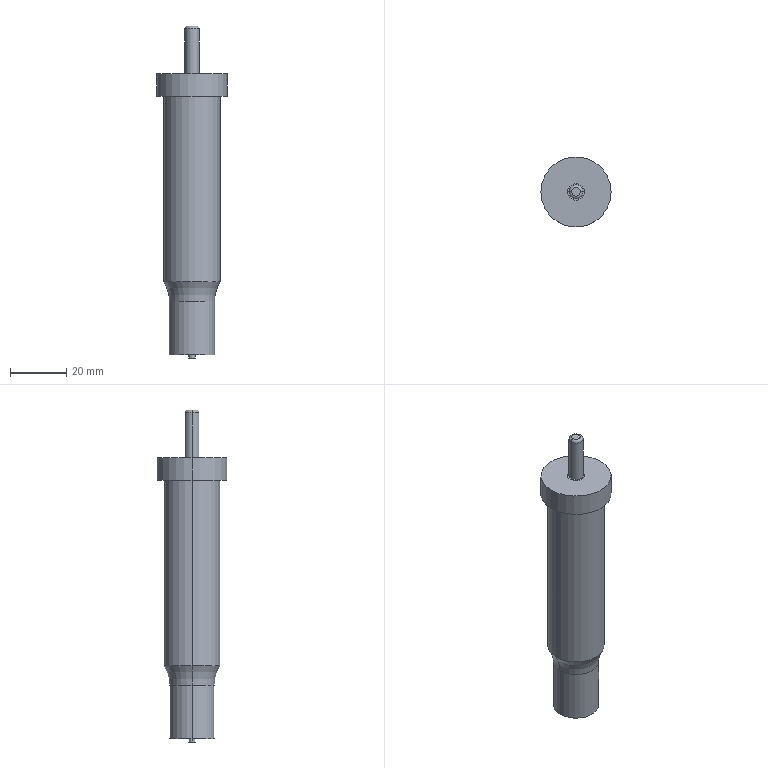Part | STEP file | 1_id3662_x_t | 1 solid | 22 faces | box 25 x 25 x 118.2 mm | volume 30521 mm3 | cylinder 12 | plane 6 | torus 4 | commonest cylinder face diameters 2.26 x2 5 x2 6 x2 16.07 x2 20 x2 25 x2
STEP:
#1=CARTESIAN_POINT('',(3377.,75.5,84.5));
#2=VERTEX_POINT('',#1);
#3=CARTESIAN_POINT('',(3377.,75.5,92.5));
#4=VERTEX_POINT('',#3);
#5=CARTESIAN_POINT('',(3377.,75.5,88.5));
#6=DIRECTION('',(0.,0.,1.));
#7=VECTOR('',#6,1.);
#8=LINE('',#5,#7);
#9=EDGE_CURVE('',#2,#4,#8,.T.);
#10=ORIENTED_EDGE('',*,*,#9,.F.);
#11=CARTESIAN_POINT('',(3352.,75.5,84.5));
#12=VERTEX_POINT('',#11);
#13=CARTESIAN_POINT('',(3364.5,75.5,84.5));
#14=DIRECTION('',(0.,0.,1.));
#15=DIRECTION('',(1.,0.,0.));
#16=AXIS2_PLACEMENT_3D('',#13,#14,#15);
#17=CIRCLE('',#16,12.5);
#18=EDGE_CURVE('',#2,#12,#17,.T.);
#19=ORIENTED_EDGE('',*,*,#18,.T.);
#20=CARTESIAN_POINT('',(3352.,75.5,92.5));
#21=VERTEX_POINT('',#20);
#22=CARTESIAN_POINT('',(3352.,75.5,88.5));
#23=DIRECTION('',(0.,0.,-1.));
#24=VECTOR('',#23,1.);
#25=LINE('',#22,#24);
#26=EDGE_CURVE('',#21,#12,#25,.T.);
#27=ORIENTED_EDGE('',*,*,#26,.F.);
#28=CARTESIAN_POINT('',(3364.5,75.5,92.5));
#29=DIRECTION('',(0.,0.,1.));
#30=DIRECTION('',(1.,0.,0.));
#31=AXIS2_PLACEMENT_3D('',#28,#29,#30);
#32=CIRCLE('',#31,12.5);
#33=EDGE_CURVE('',#4,#21,#32,.T.);
#34=ORIENTED_EDGE('',*,*,#33,.F.);
#35=EDGE_LOOP('',(#10,#19,#27,#34));
#36=FACE_OUTER_BOUND('',#35,.T.);
#37=CARTESIAN_POINT('',(3364.5,75.5,88.5));
#38=DIRECTION('',(0.,0.,-1.));
#39=DIRECTION('',(-1.,0.,0.));
#40=AXIS2_PLACEMENT_3D('',#37,#38,#39);
#41=CYLINDRICAL_SURFACE('',#40,12.5);
#42=ADVANCED_FACE('',(#36),#41,.T.);
#43=CARTESIAN_POINT('',(3374.5,75.5,18.372));
#44=VERTEX_POINT('',#43);
#45=CARTESIAN_POINT('',(3374.5,75.5,84.5));
#46=VERTEX_POINT('',#45);
#47=CARTESIAN_POINT('',(3374.5,75.5,38.5));
#48=DIRECTION('',(0.,0.,1.));
#49=VECTOR('',#48,1.);
#50=LINE('',#47,#49);
#51=EDGE_CURVE('',#44,#46,#50,.T.);
#52=ORIENTED_EDGE('',*,*,#51,.F.);
#53=CARTESIAN_POINT('',(3354.5,75.5,18.372));
#54=VERTEX_POINT('',#53);
#55=CARTESIAN_POINT('',(3364.5,75.5,18.372));
#56=DIRECTION('',(0.,0.,1.));
#57=DIRECTION('',(1.,0.,0.));
#58=AXIS2_PLACEMENT_3D('',#55,#56,#57);
#59=CIRCLE('',#58,10.);
#60=EDGE_CURVE('',#44,#54,#59,.T.);
#61=ORIENTED_EDGE('',*,*,#60,.T.);
#62=CARTESIAN_POINT('',(3354.5,75.5,84.5));
#63=VERTEX_POINT('',#62);
#64=CARTESIAN_POINT('',(3354.5,75.5,38.5));
#65=DIRECTION('',(0.,0.,-1.));
#66=VECTOR('',#65,1.);
#67=LINE('',#64,#66);
#68=EDGE_CURVE('',#63,#54,#67,.T.);
#69=ORIENTED_EDGE('',*,*,#68,.F.);
#70=CARTESIAN_POINT('',(3364.5,75.5,84.5));
#71=DIRECTION('',(0.,0.,1.));
#72=DIRECTION('',(1.,0.,0.));
#73=AXIS2_PLACEMENT_3D('',#70,#71,#72);
#74=CIRCLE('',#73,10.);
#75=EDGE_CURVE('',#46,#63,#74,.T.);
#76=ORIENTED_EDGE('',*,*,#75,.F.);
#77=EDGE_LOOP('',(#52,#61,#69,#76));
#78=FACE_OUTER_BOUND('',#77,.T.);
#79=CARTESIAN_POINT('',(3364.5,75.5,38.5));
#80=DIRECTION('',(0.,0.,-1.));
#81=DIRECTION('',(-1.,0.,0.));
#82=AXIS2_PLACEMENT_3D('',#79,#80,#81);
#83=CYLINDRICAL_SURFACE('',#82,10.);
#84=ADVANCED_FACE('',(#78),#83,.T.);
#85=CARTESIAN_POINT('',(3372.535,75.5,11.5));
#86=VERTEX_POINT('',#85);
#87=CARTESIAN_POINT('',(3372.535,75.5,-7.5));
#88=VERTEX_POINT('',#87);
#89=CARTESIAN_POINT('',(3372.535,75.5,2.));
#90=DIRECTION('',(0.,0.,-1.));
#91=VECTOR('',#90,1.);
#92=LINE('',#89,#91);
#93=EDGE_CURVE('',#86,#88,#92,.T.);
#94=ORIENTED_EDGE('',*,*,#93,.F.);
#95=CARTESIAN_POINT('',(3356.465,75.5,11.5));
#96=VERTEX_POINT('',#95);
#97=CARTESIAN_POINT('',(3364.5,75.5,11.5));
#98=DIRECTION('',(0.,0.,1.));
#99=DIRECTION('',(1.,0.,0.));
#100=AXIS2_PLACEMENT_3D('',#97,#98,#99);
#101=CIRCLE('',#100,8.035);
#102=EDGE_CURVE('',#96,#86,#101,.T.);
#103=ORIENTED_EDGE('',*,*,#102,.F.);
#104=CARTESIAN_POINT('',(3356.465,75.5,-7.5));
#105=VERTEX_POINT('',#104);
#106=CARTESIAN_POINT('',(3356.465,75.5,2.));
#107=DIRECTION('',(0.,0.,1.));
#108=VECTOR('',#107,1.);
#109=LINE('',#106,#108);
#110=EDGE_CURVE('',#105,#96,#109,.T.);
#111=ORIENTED_EDGE('',*,*,#110,.F.);
#112=CARTESIAN_POINT('',(3364.5,75.5,-7.5));
#113=DIRECTION('',(0.,0.,-1.));
#114=DIRECTION('',(1.,0.,0.));
#115=AXIS2_PLACEMENT_3D('',#112,#113,#114);
#116=CIRCLE('',#115,8.035);
#117=EDGE_CURVE('',#88,#105,#116,.T.);
#118=ORIENTED_EDGE('',*,*,#117,.F.);
#119=EDGE_LOOP('',(#94,#103,#111,#118));
#120=FACE_OUTER_BOUND('',#119,.T.);
#121=CARTESIAN_POINT('',(3364.5,75.5,2.));
#122=DIRECTION('',(0.,0.,-1.));
#123=DIRECTION('',(-1.,0.,0.));
#124=AXIS2_PLACEMENT_3D('',#121,#122,#123);
#125=CYLINDRICAL_SURFACE('',#124,8.035);
#126=ADVANCED_FACE('',(#120),#125,.T.);
#127=CARTESIAN_POINT('',(3343.465,75.5,11.5));
#128=DIRECTION('',(0.,-1.,0.));
#129=DIRECTION('',(-1.,0.,0.));
#130=AXIS2_PLACEMENT_3D('',#127,#128,#129);
#131=CIRCLE('',#130,13.);
#132=EDGE_CURVE('',#96,#54,#131,.T.);
#133=ORIENTED_EDGE('',*,*,#132,.F.);
#134=ORIENTED_EDGE('',*,*,#102,.T.);
#135=CARTESIAN_POINT('',(3385.535,75.5,11.5));
#136=DIRECTION('',(0.,-1.,0.));
#137=DIRECTION('',(1.,0.,0.));
#138=AXIS2_PLACEMENT_3D('',#135,#136,#137);
#139=CIRCLE('',#138,13.);
#140=EDGE_CURVE('',#44,#86,#139,.T.);
#141=ORIENTED_EDGE('',*,*,#140,.F.);
#142=CARTESIAN_POINT('',(3364.5,75.5,18.372));
#143=DIRECTION('',(0.,0.,1.));
#144=DIRECTION('',(1.,0.,0.));
#145=AXIS2_PLACEMENT_3D('',#142,#143,#144);
#146=CIRCLE('',#145,10.);
#147=EDGE_CURVE('',#54,#44,#146,.T.);
#148=ORIENTED_EDGE('',*,*,#147,.F.);
#149=EDGE_LOOP('',(#133,#134,#141,#148));
#150=FACE_OUTER_BOUND('',#149,.T.);
#151=CARTESIAN_POINT('',(3364.5,75.5,11.5));
#152=DIRECTION('',(0.,0.,1.));
#153=DIRECTION('',(1.,0.,0.));
#154=AXIS2_PLACEMENT_3D('',#151,#152,#153);
#155=TOROIDAL_SURFACE('',#154,21.035,13.);
#156=ADVANCED_FACE('',(#150),#155,.F.);
#157=CARTESIAN_POINT('',(3363.37,75.5,-7.5));
#158=VERTEX_POINT('',#157);
#159=CARTESIAN_POINT('',(3363.37,75.5,-8.7));
#160=VERTEX_POINT('',#159);
#161=CARTESIAN_POINT('',(3363.37,75.5,-7.5));
#162=DIRECTION('',(0.,0.,-1.));
#163=VECTOR('',#162,1.);
#164=LINE('',#161,#163);
#165=EDGE_CURVE('',#158,#160,#164,.T.);
#166=ORIENTED_EDGE('',*,*,#165,.F.);
#167=CARTESIAN_POINT('',(3365.63,75.5,-7.5));
#168=VERTEX_POINT('',#167);
#169=CARTESIAN_POINT('',(3364.5,75.5,-7.5));
#170=DIRECTION('',(0.,0.,1.));
#171=DIRECTION('',(-1.,0.,0.));
#172=AXIS2_PLACEMENT_3D('',#169,#170,#171);
#173=CIRCLE('',#172,1.13);
#174=EDGE_CURVE('',#168,#158,#173,.T.);
#175=ORIENTED_EDGE('',*,*,#174,.F.);
#176=CARTESIAN_POINT('',(3365.63,75.5,-8.7));
#177=VERTEX_POINT('',#176);
#178=CARTESIAN_POINT('',(3365.63,75.5,-7.5));
#179=DIRECTION('',(0.,0.,1.));
#180=VECTOR('',#179,1.);
#181=LINE('',#178,#180);
#182=EDGE_CURVE('',#177,#168,#181,.T.);
#183=ORIENTED_EDGE('',*,*,#182,.F.);
#184=CARTESIAN_POINT('',(3364.5,75.5,-8.7));
#185=DIRECTION('',(0.,0.,1.));
#186=DIRECTION('',(-1.,0.,0.));
#187=AXIS2_PLACEMENT_3D('',#184,#185,#186);
#188=CIRCLE('',#187,1.13);
#189=EDGE_CURVE('',#177,#160,#188,.T.);
#190=ORIENTED_EDGE('',*,*,#189,.T.);
#191=EDGE_LOOP('',(#166,#175,#183,#190));
#192=FACE_OUTER_BOUND('',#191,.T.);
#193=CARTESIAN_POINT('',(3364.5,75.5,-7.5));
#194=DIRECTION('',(0.,0.,1.));
#195=DIRECTION('',(1.,0.,0.));
#196=AXIS2_PLACEMENT_3D('',#193,#194,#195);
#197=CYLINDRICAL_SURFACE('',#196,1.13);
#198=ADVANCED_FACE('',(#192),#197,.T.);
#199=CARTESIAN_POINT('',(3362.,75.5,108.5));
#200=VERTEX_POINT('',#199);
#201=CARTESIAN_POINT('',(3362.,75.5,92.6));
#202=VERTEX_POINT('',#201);
#203=CARTESIAN_POINT('',(3362.,75.5,100.55));
#204=DIRECTION('',(0.,0.,-1.));
#205=VECTOR('',#204,1.);
#206=LINE('',#203,#205);
#207=EDGE_CURVE('',#200,#202,#206,.T.);
#208=ORIENTED_EDGE('',*,*,#207,.F.);
#209=CARTESIAN_POINT('',(3367.,75.5,108.5));
#210=VERTEX_POINT('',#209);
#211=CARTESIAN_POINT('',(3364.5,75.5,108.5));
#212=DIRECTION('',(0.,0.,-1.));
#213=DIRECTION('',(-1.,0.,0.));
#214=AXIS2_PLACEMENT_3D('',#211,#212,#213);
#215=CIRCLE('',#214,2.5);
#216=EDGE_CURVE('',#200,#210,#215,.T.);
#217=ORIENTED_EDGE('',*,*,#216,.T.);
#218=CARTESIAN_POINT('',(3367.,75.5,92.6));
#219=VERTEX_POINT('',#218);
#220=CARTESIAN_POINT('',(3367.,75.5,100.55));
#221=DIRECTION('',(0.,0.,1.));
#222=VECTOR('',#221,1.);
#223=LINE('',#220,#222);
#224=EDGE_CURVE('',#219,#210,#223,.T.);
#225=ORIENTED_EDGE('',*,*,#224,.F.);
#226=CARTESIAN_POINT('',(3364.5,75.5,92.6));
#227=DIRECTION('',(0.,0.,-1.));
#228=DIRECTION('',(-1.,0.,0.));
#229=AXIS2_PLACEMENT_3D('',#226,#227,#228);
#230=CIRCLE('',#229,2.5);
#231=EDGE_CURVE('',#202,#219,#230,.T.);
#232=ORIENTED_EDGE('',*,*,#231,.F.);
#233=EDGE_LOOP('',(#208,#217,#225,#232));
#234=FACE_OUTER_BOUND('',#233,.T.);
#235=CARTESIAN_POINT('',(3364.5,75.5,100.55));
#236=DIRECTION('',(0.,0.,1.));
#237=DIRECTION('',(1.,0.,0.));
#238=AXIS2_PLACEMENT_3D('',#235,#236,#237);
#239=CYLINDRICAL_SURFACE('',#238,2.5);
#240=ADVANCED_FACE('',(#234),#239,.T.);
#241=CARTESIAN_POINT('',(3366.,75.5,109.5));
#242=VERTEX_POINT('',#241);
#243=CARTESIAN_POINT('',(3366.,75.5,108.5));
#244=DIRECTION('',(0.,1.,0.));
#245=DIRECTION('',(1.,0.,0.));
#246=AXIS2_PLACEMENT_3D('',#243,#244,#245);
#247=CIRCLE('',#246,1.);
#248=EDGE_CURVE('',#242,#210,#247,.T.);
#249=ORIENTED_EDGE('',*,*,#248,.F.);
#250=CARTESIAN_POINT('',(3363.,75.5,109.5));
#251=VERTEX_POINT('',#250);
#252=CARTESIAN_POINT('',(3364.5,75.5,109.5));
#253=DIRECTION('',(0.,0.,-1.));
#254=DIRECTION('',(-1.,0.,0.));
#255=AXIS2_PLACEMENT_3D('',#252,#253,#254);
#256=CIRCLE('',#255,1.5);
#257=EDGE_CURVE('',#242,#251,#256,.T.);
#258=ORIENTED_EDGE('',*,*,#257,.T.);
#259=CARTESIAN_POINT('',(3363.,75.5,108.5));
#260=DIRECTION('',(0.,1.,0.));
#261=DIRECTION('',(-1.,0.,0.));
#262=AXIS2_PLACEMENT_3D('',#259,#260,#261);
#263=CIRCLE('',#262,1.);
#264=EDGE_CURVE('',#200,#251,#263,.T.);
#265=ORIENTED_EDGE('',*,*,#264,.F.);
#266=CARTESIAN_POINT('',(3364.5,75.5,108.5));
#267=DIRECTION('',(0.,0.,-1.));
#268=DIRECTION('',(-1.,0.,0.));
#269=AXIS2_PLACEMENT_3D('',#266,#267,#268);
#270=CIRCLE('',#269,2.5);
#271=EDGE_CURVE('',#210,#200,#270,.T.);
#272=ORIENTED_EDGE('',*,*,#271,.F.);
#273=EDGE_LOOP('',(#249,#258,#265,#272));
#274=FACE_OUTER_BOUND('',#273,.T.);
#275=CARTESIAN_POINT('',(3364.5,75.5,108.5));
#276=DIRECTION('',(0.,0.,-1.));
#277=DIRECTION('',(-1.,0.,0.));
#278=AXIS2_PLACEMENT_3D('',#275,#276,#277);
#279=TOROIDAL_SURFACE('',#278,1.5,1.);
#280=ADVANCED_FACE('',(#274),#279,.T.);
#281=CARTESIAN_POINT('',(3361.5,75.5,92.6));
#282=VERTEX_POINT('',#281);
#283=CARTESIAN_POINT('',(3361.5,75.5,92.5));
#284=VERTEX_POINT('',#283);
#285=CARTESIAN_POINT('',(3361.5,75.5,92.55));
#286=DIRECTION('',(0.,0.,-1.));
#287=VECTOR('',#286,1.);
#288=LINE('',#285,#287);
#289=EDGE_CURVE('',#282,#284,#288,.T.);
#290=ORIENTED_EDGE('',*,*,#289,.F.);
#291=CARTESIAN_POINT('',(3367.5,75.5,92.6));
#292=VERTEX_POINT('',#291);
#293=CARTESIAN_POINT('',(3364.5,75.5,92.6));
#294=DIRECTION('',(0.,0.,-1.));
#295=DIRECTION('',(-1.,0.,0.));
#296=AXIS2_PLACEMENT_3D('',#293,#294,#295);
#297=CIRCLE('',#296,3.);
#298=EDGE_CURVE('',#282,#292,#297,.T.);
#299=ORIENTED_EDGE('',*,*,#298,.T.);
#300=CARTESIAN_POINT('',(3367.5,75.5,92.5));
#301=VERTEX_POINT('',#300);
#302=CARTESIAN_POINT('',(3367.5,75.5,92.55));
#303=DIRECTION('',(0.,0.,1.));
#304=VECTOR('',#303,1.);
#305=LINE('',#302,#304);
#306=EDGE_CURVE('',#301,#292,#305,.T.);
#307=ORIENTED_EDGE('',*,*,#306,.F.);
#308=CARTESIAN_POINT('',(3364.5,75.5,92.5));
#309=DIRECTION('',(0.,0.,-1.));
#310=DIRECTION('',(-1.,0.,0.));
#311=AXIS2_PLACEMENT_3D('',#308,#309,#310);
#312=CIRCLE('',#311,3.);
#313=EDGE_CURVE('',#284,#301,#312,.T.);
#314=ORIENTED_EDGE('',*,*,#313,.F.);
#315=EDGE_LOOP('',(#290,#299,#307,#314));
#316=FACE_OUTER_BOUND('',#315,.T.);
#317=CARTESIAN_POINT('',(3364.5,75.5,87.05));
#318=DIRECTION('',(0.,0.,1.));
#319=DIRECTION('',(1.,0.,0.));
#320=AXIS2_PLACEMENT_3D('',#317,#318,#319);
#321=CYLINDRICAL_SURFACE('',#320,3.);
#322=ADVANCED_FACE('',(#316),#321,.T.);
#323=ORIENTED_EDGE('',*,*,#289,.T.);
#324=CARTESIAN_POINT('',(3364.5,75.5,92.5));
#325=DIRECTION('',(0.,0.,-1.));
#326=DIRECTION('',(-1.,0.,0.));
#327=AXIS2_PLACEMENT_3D('',#324,#325,#326);
#328=CIRCLE('',#327,3.);
#329=EDGE_CURVE('',#301,#284,#328,.T.);
#330=ORIENTED_EDGE('',*,*,#329,.F.);
#331=ORIENTED_EDGE('',*,*,#306,.T.);
#332=CARTESIAN_POINT('',(3364.5,75.5,92.6));
#333=DIRECTION('',(0.,0.,-1.));
#334=DIRECTION('',(-1.,0.,0.));
#335=AXIS2_PLACEMENT_3D('',#332,#333,#334);
#336=CIRCLE('',#335,3.);
#337=EDGE_CURVE('',#292,#282,#336,.T.);
#338=ORIENTED_EDGE('',*,*,#337,.T.);
#339=EDGE_LOOP('',(#323,#330,#331,#338));
#340=FACE_OUTER_BOUND('',#339,.T.);
#341=CARTESIAN_POINT('',(3364.5,75.5,87.05));
#342=DIRECTION('',(0.,0.,1.));
#343=DIRECTION('',(1.,0.,0.));
#344=AXIS2_PLACEMENT_3D('',#341,#342,#343);
#345=CYLINDRICAL_SURFACE('',#344,3.);
#346=ADVANCED_FACE('',(#340),#345,.T.);
#347=CARTESIAN_POINT('',(3364.5,75.5,109.5));
#348=DIRECTION('',(0.,0.,-1.));
#349=DIRECTION('',(-1.,0.,0.));
#350=AXIS2_PLACEMENT_3D('',#347,#348,#349);
#351=CIRCLE('',#350,1.5);
#352=EDGE_CURVE('',#251,#242,#351,.T.);
#353=ORIENTED_EDGE('',*,*,#352,.F.);
#354=ORIENTED_EDGE('',*,*,#257,.F.);
#355=EDGE_LOOP('',(#353,#354));
#356=FACE_OUTER_BOUND('',#355,.T.);
#357=CARTESIAN_POINT('',(3363.75,75.5,109.5));
#358=DIRECTION('',(0.,0.,1.));
#359=DIRECTION('',(-1.,0.,0.));
#360=AXIS2_PLACEMENT_3D('',#357,#358,#359);
#361=PLANE('',#360);
#362=ADVANCED_FACE('',(#356),#361,.T.);
#363=ORIENTED_EDGE('',*,*,#248,.T.);
#364=ORIENTED_EDGE('',*,*,#216,.F.);
#365=ORIENTED_EDGE('',*,*,#264,.T.);
#366=ORIENTED_EDGE('',*,*,#352,.T.);
#367=EDGE_LOOP('',(#363,#364,#365,#366));
#368=FACE_OUTER_BOUND('',#367,.T.);
#369=CARTESIAN_POINT('',(3364.5,75.5,108.5));
#370=DIRECTION('',(0.,0.,-1.));
#371=DIRECTION('',(-1.,0.,0.));
#372=AXIS2_PLACEMENT_3D('',#369,#370,#371);
#373=TOROIDAL_SURFACE('',#372,1.5,1.);
#374=ADVANCED_FACE('',(#368),#373,.T.);
#375=ORIENTED_EDGE('',*,*,#207,.T.);
#376=CARTESIAN_POINT('',(3364.5,75.5,92.6));
#377=DIRECTION('',(0.,0.,-1.));
#378=DIRECTION('',(-1.,0.,0.));
#379=AXIS2_PLACEMENT_3D('',#376,#377,#378);
#380=CIRCLE('',#379,2.5);
#381=EDGE_CURVE('',#219,#202,#380,.T.);
#382=ORIENTED_EDGE('',*,*,#381,.F.);
#383=ORIENTED_EDGE('',*,*,#224,.T.);
#384=ORIENTED_EDGE('',*,*,#271,.T.);
#385=EDGE_LOOP('',(#375,#382,#383,#384));
#386=FACE_OUTER_BOUND('',#385,.T.);
#387=CARTESIAN_POINT('',(3364.5,75.5,100.55));
#388=DIRECTION('',(0.,0.,1.));
#389=DIRECTION('',(1.,0.,0.));
#390=AXIS2_PLACEMENT_3D('',#387,#388,#389);
#391=CYLINDRICAL_SURFACE('',#390,2.5);
#392=ADVANCED_FACE('',(#386),#391,.T.);
#393=ORIENTED_EDGE('',*,*,#298,.F.);
#394=ORIENTED_EDGE('',*,*,#337,.F.);
#395=EDGE_LOOP('',(#393,#394));
#396=FACE_BOUND('',#395,.T.);
#397=ORIENTED_EDGE('',*,*,#231,.T.);
#398=ORIENTED_EDGE('',*,*,#381,.T.);
#399=EDGE_LOOP('',(#397,#398));
#400=FACE_BOUND('',#399,.T.);
#401=CARTESIAN_POINT('',(3361.75,75.5,92.6));
#402=DIRECTION('',(0.,0.,1.));
#403=DIRECTION('',(-1.,0.,0.));
#404=AXIS2_PLACEMENT_3D('',#401,#402,#403);
#405=PLANE('',#404);
#406=ADVANCED_FACE('',(#396,#400),#405,.T.);
#407=ORIENTED_EDGE('',*,*,#165,.T.);
#408=CARTESIAN_POINT('',(3364.5,75.5,-8.7));
#409=DIRECTION('',(0.,0.,1.));
#410=DIRECTION('',(-1.,0.,0.));
#411=AXIS2_PLACEMENT_3D('',#408,#409,#410);
#412=CIRCLE('',#411,1.13);
#413=EDGE_CURVE('',#160,#177,#412,.T.);
#414=ORIENTED_EDGE('',*,*,#413,.T.);
#415=ORIENTED_EDGE('',*,*,#182,.T.);
#416=CARTESIAN_POINT('',(3364.5,75.5,-7.5));
#417=DIRECTION('',(0.,0.,1.));
#418=DIRECTION('',(-1.,0.,0.));
#419=AXIS2_PLACEMENT_3D('',#416,#417,#418);
#420=CIRCLE('',#419,1.13);
#421=EDGE_CURVE('',#158,#168,#420,.T.);
#422=ORIENTED_EDGE('',*,*,#421,.F.);
#423=EDGE_LOOP('',(#407,#414,#415,#422));
#424=FACE_OUTER_BOUND('',#423,.T.);
#425=CARTESIAN_POINT('',(3364.5,75.5,-7.5));
#426=DIRECTION('',(0.,0.,1.));
#427=DIRECTION('',(1.,0.,0.));
#428=AXIS2_PLACEMENT_3D('',#425,#426,#427);
#429=CYLINDRICAL_SURFACE('',#428,1.13);
#430=ADVANCED_FACE('',(#424),#429,.T.);
#431=ORIENTED_EDGE('',*,*,#413,.F.);
#432=ORIENTED_EDGE('',*,*,#189,.F.);
#433=EDGE_LOOP('',(#431,#432));
#434=FACE_OUTER_BOUND('',#433,.T.);
#435=CARTESIAN_POINT('',(3364.5,75.5,-8.7));
#436=DIRECTION('',(0.,0.,1.));
#437=DIRECTION('',(1.,0.,0.));
#438=AXIS2_PLACEMENT_3D('',#435,#436,#437);
#439=PLANE('',#438);
#440=ADVANCED_FACE('',(#434),#439,.F.);
#441=ORIENTED_EDGE('',*,*,#132,.T.);
#442=ORIENTED_EDGE('',*,*,#60,.F.);
#443=ORIENTED_EDGE('',*,*,#140,.T.);
#444=CARTESIAN_POINT('',(3364.5,75.5,11.5));
#445=DIRECTION('',(0.,0.,1.));
#446=DIRECTION('',(1.,0.,0.));
#447=AXIS2_PLACEMENT_3D('',#444,#445,#446);
#448=CIRCLE('',#447,8.035);
#449=EDGE_CURVE('',#86,#96,#448,.T.);
#450=ORIENTED_EDGE('',*,*,#449,.T.);
#451=EDGE_LOOP('',(#441,#442,#443,#450));
#452=FACE_OUTER_BOUND('',#451,.T.);
#453=CARTESIAN_POINT('',(3364.5,75.5,11.5));
#454=DIRECTION('',(0.,0.,1.));
#455=DIRECTION('',(1.,0.,0.));
#456=AXIS2_PLACEMENT_3D('',#453,#454,#455);
#457=TOROIDAL_SURFACE('',#456,21.035,13.);
#458=ADVANCED_FACE('',(#452),#457,.F.);
#459=ORIENTED_EDGE('',*,*,#93,.T.);
#460=CARTESIAN_POINT('',(3364.5,75.5,-7.5));
#461=DIRECTION('',(0.,0.,-1.));
#462=DIRECTION('',(1.,0.,0.));
#463=AXIS2_PLACEMENT_3D('',#460,#461,#462);
#464=CIRCLE('',#463,8.035);
#465=EDGE_CURVE('',#105,#88,#464,.T.);
#466=ORIENTED_EDGE('',*,*,#465,.F.);
#467=ORIENTED_EDGE('',*,*,#110,.T.);
#468=ORIENTED_EDGE('',*,*,#449,.F.);
#469=EDGE_LOOP('',(#459,#466,#467,#468));
#470=FACE_OUTER_BOUND('',#469,.T.);
#471=CARTESIAN_POINT('',(3364.5,75.5,2.));
#472=DIRECTION('',(0.,0.,-1.));
#473=DIRECTION('',(-1.,0.,0.));
#474=AXIS2_PLACEMENT_3D('',#471,#472,#473);
#475=CYLINDRICAL_SURFACE('',#474,8.035);
#476=ADVANCED_FACE('',(#470),#475,.T.);
#477=ORIENTED_EDGE('',*,*,#421,.T.);
#478=ORIENTED_EDGE('',*,*,#174,.T.);
#479=EDGE_LOOP('',(#477,#478));
#480=FACE_BOUND('',#479,.T.);
#481=ORIENTED_EDGE('',*,*,#117,.T.);
#482=ORIENTED_EDGE('',*,*,#465,.T.);
#483=EDGE_LOOP('',(#481,#482));
#484=FACE_BOUND('',#483,.T.);
#485=CARTESIAN_POINT('',(3369.5,75.5,-7.5));
#486=DIRECTION('',(0.,0.,-1.));
#487=DIRECTION('',(1.,0.,0.));
#488=AXIS2_PLACEMENT_3D('',#485,#486,#487);
#489=PLANE('',#488);
#490=ADVANCED_FACE('',(#480,#484),#489,.T.);
#491=ORIENTED_EDGE('',*,*,#51,.T.);
#492=CARTESIAN_POINT('',(3364.5,75.5,84.5));
#493=DIRECTION('',(0.,0.,1.));
#494=DIRECTION('',(1.,0.,0.));
#495=AXIS2_PLACEMENT_3D('',#492,#493,#494);
#496=CIRCLE('',#495,10.);
#497=EDGE_CURVE('',#63,#46,#496,.T.);
#498=ORIENTED_EDGE('',*,*,#497,.F.);
#499=ORIENTED_EDGE('',*,*,#68,.T.);
#500=ORIENTED_EDGE('',*,*,#147,.T.);
#501=EDGE_LOOP('',(#491,#498,#499,#500));
#502=FACE_OUTER_BOUND('',#501,.T.);
#503=CARTESIAN_POINT('',(3364.5,75.5,38.5));
#504=DIRECTION('',(0.,0.,-1.));
#505=DIRECTION('',(-1.,0.,0.));
#506=AXIS2_PLACEMENT_3D('',#503,#504,#505);
#507=CYLINDRICAL_SURFACE('',#506,10.);
#508=ADVANCED_FACE('',(#502),#507,.T.);
#509=ORIENTED_EDGE('',*,*,#18,.F.);
#510=CARTESIAN_POINT('',(3364.5,75.5,84.5));
#511=DIRECTION('',(0.,0.,1.));
#512=DIRECTION('',(1.,0.,0.));
#513=AXIS2_PLACEMENT_3D('',#510,#511,#512);
#514=CIRCLE('',#513,12.5);
#515=EDGE_CURVE('',#12,#2,#514,.T.);
#516=ORIENTED_EDGE('',*,*,#515,.F.);
#517=EDGE_LOOP('',(#509,#516));
#518=FACE_BOUND('',#517,.T.);
#519=ORIENTED_EDGE('',*,*,#75,.T.);
#520=ORIENTED_EDGE('',*,*,#497,.T.);
#521=EDGE_LOOP('',(#519,#520));
#522=FACE_BOUND('',#521,.T.);
#523=CARTESIAN_POINT('',(3375.75,75.5,84.5));
#524=DIRECTION('',(0.,0.,-1.));
#525=DIRECTION('',(1.,0.,0.));
#526=AXIS2_PLACEMENT_3D('',#523,#524,#525);
#527=PLANE('',#526);
#528=ADVANCED_FACE('',(#518,#522),#527,.T.);
#529=ORIENTED_EDGE('',*,*,#9,.T.);
#530=CARTESIAN_POINT('',(3364.5,75.5,92.5));
#531=DIRECTION('',(0.,0.,1.));
#532=DIRECTION('',(1.,0.,0.));
#533=AXIS2_PLACEMENT_3D('',#530,#531,#532);
#534=CIRCLE('',#533,12.5);
#535=EDGE_CURVE('',#21,#4,#534,.T.);
#536=ORIENTED_EDGE('',*,*,#535,.F.);
#537=ORIENTED_EDGE('',*,*,#26,.T.);
#538=ORIENTED_EDGE('',*,*,#515,.T.);
#539=EDGE_LOOP('',(#529,#536,#537,#538));
#540=FACE_OUTER_BOUND('',#539,.T.);
#541=CARTESIAN_POINT('',(3364.5,75.5,88.5));
#542=DIRECTION('',(0.,0.,-1.));
#543=DIRECTION('',(-1.,0.,0.));
#544=AXIS2_PLACEMENT_3D('',#541,#542,#543);
#545=CYLINDRICAL_SURFACE('',#544,12.5);
#546=ADVANCED_FACE('',(#540),#545,.T.);
#547=ORIENTED_EDGE('',*,*,#329,.T.);
#548=ORIENTED_EDGE('',*,*,#313,.T.);
#549=EDGE_LOOP('',(#547,#548));
#550=FACE_BOUND('',#549,.T.);
#551=ORIENTED_EDGE('',*,*,#33,.T.);
#552=ORIENTED_EDGE('',*,*,#535,.T.);
#553=EDGE_LOOP('',(#551,#552));
#554=FACE_BOUND('',#553,.T.);
#555=CARTESIAN_POINT('',(3370.75,75.5,92.5));
#556=DIRECTION('',(0.,0.,1.));
#557=DIRECTION('',(-1.,0.,0.));
#558=AXIS2_PLACEMENT_3D('',#555,#556,#557);
#559=PLANE('',#558);
#560=ADVANCED_FACE('',(#550,#554),#559,.T.);
#561=CLOSED_SHELL('',(#42,#84,#126,#156,#198,#240,#280,#322,#346,#362,#374,#392,#406,#430,#440,#458,#476,#490,#508,#528,#546,#560));
#562=MANIFOLD_SOLID_BREP('',#561);
#563=(LENGTH_UNIT()NAMED_UNIT(*)SI_UNIT(.MILLI.,.METRE.));
#564=UNCERTAINTY_MEASURE_WITH_UNIT(LENGTH_MEASURE(0.00002),#563,'','');
#565=(NAMED_UNIT(*)PLANE_ANGLE_UNIT()SI_UNIT($,.RADIAN.));
#566=PLANE_ANGLE_MEASURE_WITH_UNIT(PLANE_ANGLE_MEASURE(0.01745),#565);
#567=DIMENSIONAL_EXPONENTS(0.,0.,0.,0.,0.,0.,0.);
#568=(CONVERSION_BASED_UNIT('DEGREE',#566)NAMED_UNIT(#567)PLANE_ANGLE_UNIT());
#569=(NAMED_UNIT(*)SI_UNIT($,.STERADIAN.)SOLID_ANGLE_UNIT());
#570=(GEOMETRIC_REPRESENTATION_CONTEXT(3)GLOBAL_UNCERTAINTY_ASSIGNED_CONTEXT((#564))GLOBAL_UNIT_ASSIGNED_CONTEXT((#563,#568,#569))REPRESENTATION_CONTEXT('',''));
#571=ADVANCED_BREP_SHAPE_REPRESENTATION('',(#562),#570);